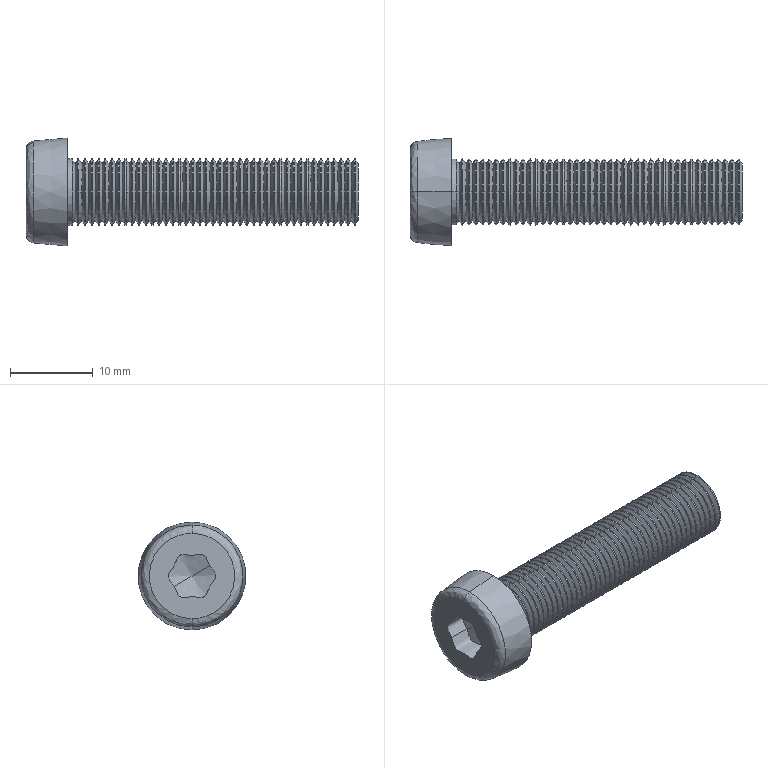Part | SolidWorks | features BaseBody 1 | 1 solid | 267 faces | box 40 x 13 x 13 mm | volume 2107 mm3 | cone 172 | cylinder 86 | spline 6 | plane 3 | commonest cylinder face diameters 8 x86